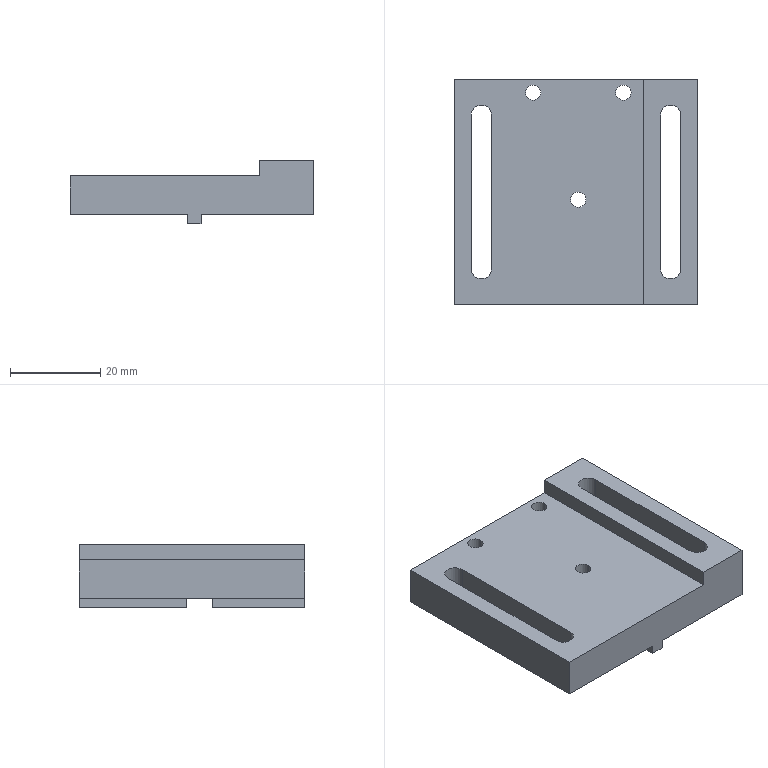Part | STEP file | ASND-0110-Camera base block | 1 solid | 40 faces | box 54 x 50 x 14 mm | volume 21543 mm3 | plane 26 | cylinder 14 | commonest cylinder face diameters 3.4 x6 4.5 x4 6.5 x4